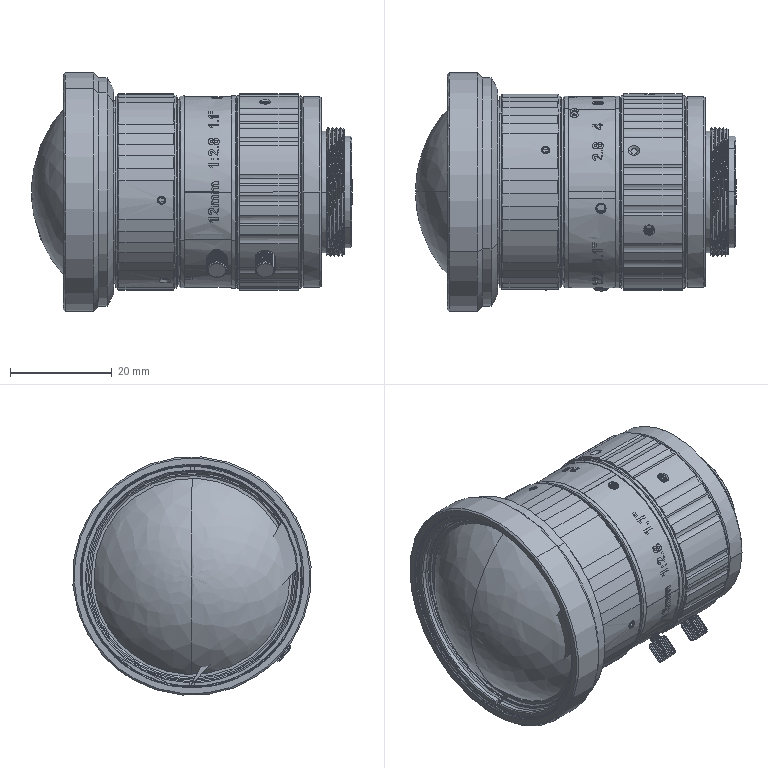Part | SolidWorks | 16 solids | 2426 faces | box 63.129 x 47 x 47 mm | volume 44730 mm3 | spline 1803 | cylinder 320 | plane 230 | cone 73 | commonest cylinder face diameters 1.6 x51 4 x36 38.6 x25 37.698 x21 31 x20 2 x18